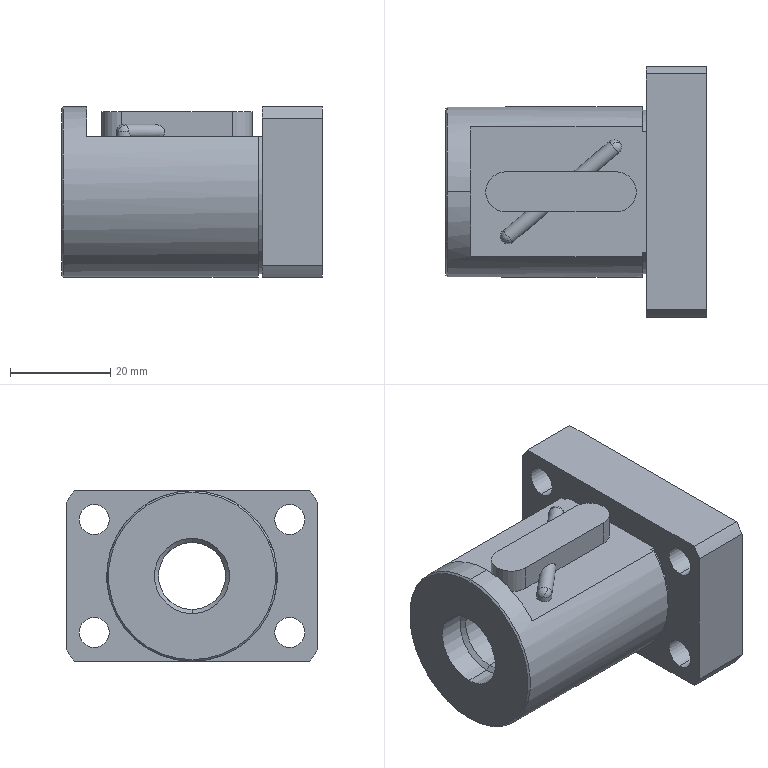Part | SolidWorks | features BaseBody 1 | 1 solid | 73 faces | box 52 x 50 x 34 mm | volume 43614 mm3 | cylinder 40 | plane 18 | sphere 8 | cone 7 | commonest cylinder face diameters 6 x8 9.5 x8 3 x4 15 x4 58 x4 4.917 x3